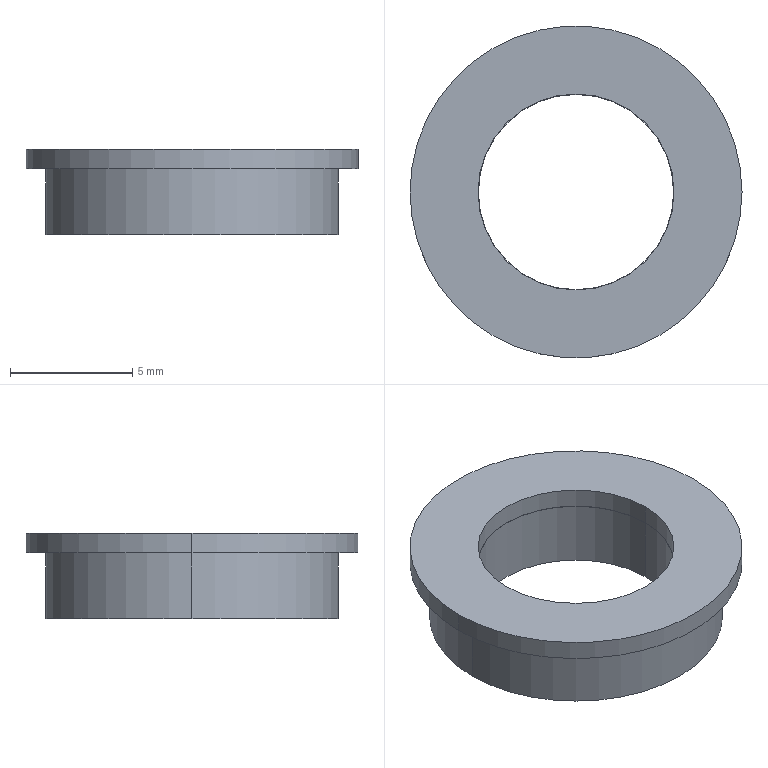Part | SolidWorks | features Extrusion 1, ICE 1 | 1 solid | 12 faces | box 13.6 x 13.6 x 3.5 mm | volume 245.378 mm3 | cylinder 8 | plane 4 | commonest cylinder face diameters 8 x2 8.027 x2 12 x2 13.6 x2
STEP:
#1=CARTESIAN_POINT('',(-4.013,0.,3.5));
#2=VERTEX_POINT('',#1);
#3=CARTESIAN_POINT('',(4.013,0.,3.5));
#4=VERTEX_POINT('',#3);
#5=CARTESIAN_POINT('',(0.,0.,3.5));
#6=DIRECTION('',(0.,0.,1.));
#7=DIRECTION('',(1.,0.,0.));
#8=AXIS2_PLACEMENT_3D('',#5,#6,#7);
#9=CIRCLE('',#8,4.013);
#10=EDGE_CURVE('',#2,#4,#9,.T.);
#11=ORIENTED_EDGE('',*,*,#10,.T.);
#12=CARTESIAN_POINT('',(4.013,0.,2.7));
#13=VERTEX_POINT('',#12);
#14=CARTESIAN_POINT('',(4.013,0.,3.5));
#15=DIRECTION('',(0.,0.,-1.));
#16=VECTOR('',#15,1000.);
#17=LINE('',#14,#16);
#18=EDGE_CURVE('',#4,#13,#17,.T.);
#19=ORIENTED_EDGE('',*,*,#18,.T.);
#20=CARTESIAN_POINT('',(-4.013,0.,2.7));
#21=VERTEX_POINT('',#20);
#22=CARTESIAN_POINT('',(0.,0.,2.7));
#23=DIRECTION('',(0.,0.,-1.));
#24=DIRECTION('',(1.,0.,0.));
#25=AXIS2_PLACEMENT_3D('',#22,#23,#24);
#26=CIRCLE('',#25,4.013);
#27=EDGE_CURVE('',#13,#21,#26,.T.);
#28=ORIENTED_EDGE('',*,*,#27,.T.);
#29=CARTESIAN_POINT('',(-4.013,0.,3.5));
#30=DIRECTION('',(0.,0.,-1.));
#31=VECTOR('',#30,1000.);
#32=LINE('',#29,#31);
#33=EDGE_CURVE('',#2,#21,#32,.T.);
#34=ORIENTED_EDGE('',*,*,#33,.F.);
#35=EDGE_LOOP('',(#11,#19,#28,#34));
#36=FACE_OUTER_BOUND('',#35,.T.);
#37=CARTESIAN_POINT('',(0.,0.,3.5));
#38=DIRECTION('',(0.,0.,-1.));
#39=DIRECTION('',(-1.,0.,0.));
#40=AXIS2_PLACEMENT_3D('',#37,#38,#39);
#41=CYLINDRICAL_SURFACE('',#40,4.013);
#42=ADVANCED_FACE('',(#36),#41,.F.);
#43=CARTESIAN_POINT('',(6.8,0.,3.5));
#44=VERTEX_POINT('',#43);
#45=CARTESIAN_POINT('',(-6.8,0.,3.5));
#46=VERTEX_POINT('',#45);
#47=CARTESIAN_POINT('',(0.,0.,3.5));
#48=DIRECTION('',(0.,0.,1.));
#49=DIRECTION('',(1.,0.,0.));
#50=AXIS2_PLACEMENT_3D('',#47,#48,#49);
#51=CIRCLE('',#50,6.8);
#52=EDGE_CURVE('',#44,#46,#51,.T.);
#53=ORIENTED_EDGE('',*,*,#52,.F.);
#54=CARTESIAN_POINT('',(6.8,0.,2.7));
#55=VERTEX_POINT('',#54);
#56=CARTESIAN_POINT('',(6.8,0.,3.5));
#57=DIRECTION('',(0.,0.,-1.));
#58=VECTOR('',#57,1000.);
#59=LINE('',#56,#58);
#60=EDGE_CURVE('',#44,#55,#59,.T.);
#61=ORIENTED_EDGE('',*,*,#60,.T.);
#62=CARTESIAN_POINT('',(-6.8,0.,2.7));
#63=VERTEX_POINT('',#62);
#64=CARTESIAN_POINT('',(0.,0.,2.7));
#65=DIRECTION('',(0.,0.,1.));
#66=DIRECTION('',(1.,0.,0.));
#67=AXIS2_PLACEMENT_3D('',#64,#65,#66);
#68=CIRCLE('',#67,6.8);
#69=EDGE_CURVE('',#55,#63,#68,.T.);
#70=ORIENTED_EDGE('',*,*,#69,.T.);
#71=CARTESIAN_POINT('',(-6.8,0.,3.5));
#72=DIRECTION('',(0.,0.,-1.));
#73=VECTOR('',#72,1000.);
#74=LINE('',#71,#73);
#75=EDGE_CURVE('',#46,#63,#74,.T.);
#76=ORIENTED_EDGE('',*,*,#75,.F.);
#77=EDGE_LOOP('',(#53,#61,#70,#76));
#78=FACE_OUTER_BOUND('',#77,.T.);
#79=CARTESIAN_POINT('',(0.,0.,3.5));
#80=DIRECTION('',(0.,0.,-1.));
#81=DIRECTION('',(-1.,0.,0.));
#82=AXIS2_PLACEMENT_3D('',#79,#80,#81);
#83=CYLINDRICAL_SURFACE('',#82,6.8);
#84=ADVANCED_FACE('',(#78),#83,.T.);
#85=CARTESIAN_POINT('',(-4.,0.,2.7));
#86=VERTEX_POINT('',#85);
#87=CARTESIAN_POINT('',(4.,0.,2.7));
#88=VERTEX_POINT('',#87);
#89=CARTESIAN_POINT('',(0.,0.,2.7));
#90=DIRECTION('',(0.,0.,1.));
#91=DIRECTION('',(1.,0.,0.));
#92=AXIS2_PLACEMENT_3D('',#89,#90,#91);
#93=CIRCLE('',#92,4.);
#94=EDGE_CURVE('',#86,#88,#93,.T.);
#95=ORIENTED_EDGE('',*,*,#94,.T.);
#96=CARTESIAN_POINT('',(4.,0.,0.));
#97=VERTEX_POINT('',#96);
#98=CARTESIAN_POINT('',(4.,0.,2.7));
#99=DIRECTION('',(0.,0.,-1.));
#100=VECTOR('',#99,1000.);
#101=LINE('',#98,#100);
#102=EDGE_CURVE('',#88,#97,#101,.T.);
#103=ORIENTED_EDGE('',*,*,#102,.T.);
#104=CARTESIAN_POINT('',(-4.,0.,0.));
#105=VERTEX_POINT('',#104);
#106=CARTESIAN_POINT('',(0.,0.,0.));
#107=DIRECTION('',(0.,0.,1.));
#108=DIRECTION('',(1.,0.,0.));
#109=AXIS2_PLACEMENT_3D('',#106,#107,#108);
#110=CIRCLE('',#109,4.);
#111=EDGE_CURVE('',#105,#97,#110,.T.);
#112=ORIENTED_EDGE('',*,*,#111,.F.);
#113=CARTESIAN_POINT('',(-4.,0.,2.7));
#114=DIRECTION('',(0.,0.,-1.));
#115=VECTOR('',#114,1000.);
#116=LINE('',#113,#115);
#117=EDGE_CURVE('',#86,#105,#116,.T.);
#118=ORIENTED_EDGE('',*,*,#117,.F.);
#119=EDGE_LOOP('',(#95,#103,#112,#118));
#120=FACE_OUTER_BOUND('',#119,.T.);
#121=CARTESIAN_POINT('',(0.,0.,2.7));
#122=DIRECTION('',(0.,0.,-1.));
#123=DIRECTION('',(-1.,0.,0.));
#124=AXIS2_PLACEMENT_3D('',#121,#122,#123);
#125=CYLINDRICAL_SURFACE('',#124,4.);
#126=ADVANCED_FACE('',(#120),#125,.F.);
#127=CARTESIAN_POINT('',(6.,0.,2.7));
#128=VERTEX_POINT('',#127);
#129=CARTESIAN_POINT('',(-6.,0.,2.7));
#130=VERTEX_POINT('',#129);
#131=CARTESIAN_POINT('',(0.,0.,2.7));
#132=DIRECTION('',(0.,0.,1.));
#133=DIRECTION('',(1.,0.,0.));
#134=AXIS2_PLACEMENT_3D('',#131,#132,#133);
#135=CIRCLE('',#134,6.);
#136=EDGE_CURVE('',#128,#130,#135,.T.);
#137=ORIENTED_EDGE('',*,*,#136,.F.);
#138=CARTESIAN_POINT('',(6.,0.,0.));
#139=VERTEX_POINT('',#138);
#140=CARTESIAN_POINT('',(6.,0.,2.7));
#141=DIRECTION('',(0.,0.,-1.));
#142=VECTOR('',#141,1000.);
#143=LINE('',#140,#142);
#144=EDGE_CURVE('',#128,#139,#143,.T.);
#145=ORIENTED_EDGE('',*,*,#144,.T.);
#146=CARTESIAN_POINT('',(-6.,0.,0.));
#147=VERTEX_POINT('',#146);
#148=CARTESIAN_POINT('',(0.,0.,0.));
#149=DIRECTION('',(0.,0.,1.));
#150=DIRECTION('',(1.,0.,0.));
#151=AXIS2_PLACEMENT_3D('',#148,#149,#150);
#152=CIRCLE('',#151,6.);
#153=EDGE_CURVE('',#139,#147,#152,.T.);
#154=ORIENTED_EDGE('',*,*,#153,.T.);
#155=CARTESIAN_POINT('',(-6.,0.,2.7));
#156=DIRECTION('',(0.,0.,-1.));
#157=VECTOR('',#156,1000.);
#158=LINE('',#155,#157);
#159=EDGE_CURVE('',#130,#147,#158,.T.);
#160=ORIENTED_EDGE('',*,*,#159,.F.);
#161=EDGE_LOOP('',(#137,#145,#154,#160));
#162=FACE_OUTER_BOUND('',#161,.T.);
#163=CARTESIAN_POINT('',(0.,0.,2.7));
#164=DIRECTION('',(0.,0.,-1.));
#165=DIRECTION('',(-1.,0.,0.));
#166=AXIS2_PLACEMENT_3D('',#163,#164,#165);
#167=CYLINDRICAL_SURFACE('',#166,6.);
#168=ADVANCED_FACE('',(#162),#167,.T.);
#169=CARTESIAN_POINT('',(0.,0.,2.7));
#170=DIRECTION('',(0.,0.,-1.));
#171=DIRECTION('',(1.,0.,0.));
#172=AXIS2_PLACEMENT_3D('',#169,#170,#171);
#173=CIRCLE('',#172,4.013);
#174=EDGE_CURVE('',#21,#13,#173,.T.);
#175=ORIENTED_EDGE('',*,*,#174,.F.);
#176=ORIENTED_EDGE('',*,*,#27,.F.);
#177=EDGE_LOOP('',(#175,#176));
#178=FACE_OUTER_BOUND('',#177,.T.);
#179=ORIENTED_EDGE('',*,*,#94,.F.);
#180=CARTESIAN_POINT('',(0.,0.,2.7));
#181=DIRECTION('',(0.,0.,1.));
#182=DIRECTION('',(1.,0.,0.));
#183=AXIS2_PLACEMENT_3D('',#180,#181,#182);
#184=CIRCLE('',#183,4.);
#185=EDGE_CURVE('',#88,#86,#184,.T.);
#186=ORIENTED_EDGE('',*,*,#185,.F.);
#187=EDGE_LOOP('',(#179,#186));
#188=FACE_BOUND('',#187,.T.);
#189=CARTESIAN_POINT('',(0.,0.,2.7));
#190=DIRECTION('',(0.,0.,1.));
#191=DIRECTION('',(1.,0.,0.));
#192=AXIS2_PLACEMENT_3D('',#189,#190,#191);
#193=PLANE('',#192);
#194=ADVANCED_FACE('',(#178,#188),#193,.T.);
#195=CARTESIAN_POINT('',(0.,0.,0.));
#196=DIRECTION('',(0.,0.,1.));
#197=DIRECTION('',(1.,0.,0.));
#198=AXIS2_PLACEMENT_3D('',#195,#196,#197);
#199=CIRCLE('',#198,6.);
#200=EDGE_CURVE('',#147,#139,#199,.T.);
#201=ORIENTED_EDGE('',*,*,#200,.F.);
#202=ORIENTED_EDGE('',*,*,#153,.F.);
#203=EDGE_LOOP('',(#201,#202));
#204=FACE_OUTER_BOUND('',#203,.T.);
#205=ORIENTED_EDGE('',*,*,#111,.T.);
#206=CARTESIAN_POINT('',(0.,0.,0.));
#207=DIRECTION('',(0.,0.,1.));
#208=DIRECTION('',(1.,0.,0.));
#209=AXIS2_PLACEMENT_3D('',#206,#207,#208);
#210=CIRCLE('',#209,4.);
#211=EDGE_CURVE('',#97,#105,#210,.T.);
#212=ORIENTED_EDGE('',*,*,#211,.T.);
#213=EDGE_LOOP('',(#205,#212));
#214=FACE_BOUND('',#213,.T.);
#215=CARTESIAN_POINT('',(0.,0.,0.));
#216=DIRECTION('',(0.,0.,1.));
#217=DIRECTION('',(1.,0.,0.));
#218=AXIS2_PLACEMENT_3D('',#215,#216,#217);
#219=PLANE('',#218);
#220=ADVANCED_FACE('',(#204,#214),#219,.F.);
#221=ORIENTED_EDGE('',*,*,#144,.F.);
#222=CARTESIAN_POINT('',(0.,0.,2.7));
#223=DIRECTION('',(0.,0.,1.));
#224=DIRECTION('',(1.,0.,0.));
#225=AXIS2_PLACEMENT_3D('',#222,#223,#224);
#226=CIRCLE('',#225,6.);
#227=EDGE_CURVE('',#130,#128,#226,.T.);
#228=ORIENTED_EDGE('',*,*,#227,.F.);
#229=ORIENTED_EDGE('',*,*,#159,.T.);
#230=ORIENTED_EDGE('',*,*,#200,.T.);
#231=EDGE_LOOP('',(#221,#228,#229,#230));
#232=FACE_OUTER_BOUND('',#231,.T.);
#233=CARTESIAN_POINT('',(0.,0.,2.7));
#234=DIRECTION('',(0.,0.,-1.));
#235=DIRECTION('',(-1.,0.,0.));
#236=AXIS2_PLACEMENT_3D('',#233,#234,#235);
#237=CYLINDRICAL_SURFACE('',#236,6.);
#238=ADVANCED_FACE('',(#232),#237,.T.);
#239=ORIENTED_EDGE('',*,*,#102,.F.);
#240=ORIENTED_EDGE('',*,*,#185,.T.);
#241=ORIENTED_EDGE('',*,*,#117,.T.);
#242=ORIENTED_EDGE('',*,*,#211,.F.);
#243=EDGE_LOOP('',(#239,#240,#241,#242));
#244=FACE_OUTER_BOUND('',#243,.T.);
#245=CARTESIAN_POINT('',(0.,0.,2.7));
#246=DIRECTION('',(0.,0.,-1.));
#247=DIRECTION('',(-1.,0.,0.));
#248=AXIS2_PLACEMENT_3D('',#245,#246,#247);
#249=CYLINDRICAL_SURFACE('',#248,4.);
#250=ADVANCED_FACE('',(#244),#249,.F.);
#251=CARTESIAN_POINT('',(0.,0.,2.7));
#252=DIRECTION('',(0.,0.,1.));
#253=DIRECTION('',(1.,0.,0.));
#254=AXIS2_PLACEMENT_3D('',#251,#252,#253);
#255=CIRCLE('',#254,6.8);
#256=EDGE_CURVE('',#63,#55,#255,.T.);
#257=ORIENTED_EDGE('',*,*,#256,.F.);
#258=ORIENTED_EDGE('',*,*,#69,.F.);
#259=EDGE_LOOP('',(#257,#258));
#260=FACE_OUTER_BOUND('',#259,.T.);
#261=ORIENTED_EDGE('',*,*,#227,.T.);
#262=ORIENTED_EDGE('',*,*,#136,.T.);
#263=EDGE_LOOP('',(#261,#262));
#264=FACE_BOUND('',#263,.T.);
#265=CARTESIAN_POINT('',(0.,0.,2.7));
#266=DIRECTION('',(0.,0.,1.));
#267=DIRECTION('',(1.,0.,0.));
#268=AXIS2_PLACEMENT_3D('',#265,#266,#267);
#269=PLANE('',#268);
#270=ADVANCED_FACE('',(#260,#264),#269,.F.);
#271=CARTESIAN_POINT('',(0.,0.,3.5));
#272=DIRECTION('',(0.,0.,1.));
#273=DIRECTION('',(1.,0.,0.));
#274=AXIS2_PLACEMENT_3D('',#271,#272,#273);
#275=CIRCLE('',#274,6.8);
#276=EDGE_CURVE('',#46,#44,#275,.T.);
#277=ORIENTED_EDGE('',*,*,#276,.T.);
#278=ORIENTED_EDGE('',*,*,#52,.T.);
#279=EDGE_LOOP('',(#277,#278));
#280=FACE_OUTER_BOUND('',#279,.T.);
#281=ORIENTED_EDGE('',*,*,#10,.F.);
#282=CARTESIAN_POINT('',(0.,0.,3.5));
#283=DIRECTION('',(0.,0.,1.));
#284=DIRECTION('',(1.,0.,0.));
#285=AXIS2_PLACEMENT_3D('',#282,#283,#284);
#286=CIRCLE('',#285,4.013);
#287=EDGE_CURVE('',#4,#2,#286,.T.);
#288=ORIENTED_EDGE('',*,*,#287,.F.);
#289=EDGE_LOOP('',(#281,#288));
#290=FACE_BOUND('',#289,.T.);
#291=CARTESIAN_POINT('',(0.,0.,3.5));
#292=DIRECTION('',(0.,0.,1.));
#293=DIRECTION('',(1.,0.,0.));
#294=AXIS2_PLACEMENT_3D('',#291,#292,#293);
#295=PLANE('',#294);
#296=ADVANCED_FACE('',(#280,#290),#295,.T.);
#297=ORIENTED_EDGE('',*,*,#60,.F.);
#298=ORIENTED_EDGE('',*,*,#276,.F.);
#299=ORIENTED_EDGE('',*,*,#75,.T.);
#300=ORIENTED_EDGE('',*,*,#256,.T.);
#301=EDGE_LOOP('',(#297,#298,#299,#300));
#302=FACE_OUTER_BOUND('',#301,.T.);
#303=CARTESIAN_POINT('',(0.,0.,3.5));
#304=DIRECTION('',(0.,0.,-1.));
#305=DIRECTION('',(-1.,0.,0.));
#306=AXIS2_PLACEMENT_3D('',#303,#304,#305);
#307=CYLINDRICAL_SURFACE('',#306,6.8);
#308=ADVANCED_FACE('',(#302),#307,.T.);
#309=ORIENTED_EDGE('',*,*,#18,.F.);
#310=ORIENTED_EDGE('',*,*,#287,.T.);
#311=ORIENTED_EDGE('',*,*,#33,.T.);
#312=ORIENTED_EDGE('',*,*,#174,.T.);
#313=EDGE_LOOP('',(#309,#310,#311,#312));
#314=FACE_OUTER_BOUND('',#313,.T.);
#315=CARTESIAN_POINT('',(0.,0.,3.5));
#316=DIRECTION('',(0.,0.,-1.));
#317=DIRECTION('',(-1.,0.,0.));
#318=AXIS2_PLACEMENT_3D('',#315,#316,#317);
#319=CYLINDRICAL_SURFACE('',#318,4.013);
#320=ADVANCED_FACE('',(#314),#319,.F.);
#321=CLOSED_SHELL('',(#42,#84,#126,#168,#194,#220,#238,#250,#270,#296,#308,#320));
#322=MANIFOLD_SOLID_BREP('',#321);
#323=CARTESIAN_POINT('',(0.,0.,0.));
#324=DIRECTION('',(0.,0.,1.));
#325=DIRECTION('',(1.,0.,0.));
#326=AXIS2_PLACEMENT_3D('',#323,#324,#325);
#327=(LENGTH_UNIT()NAMED_UNIT(*)SI_UNIT(.MILLI.,.METRE.));
#328=UNCERTAINTY_MEASURE_WITH_UNIT(LENGTH_MEASURE(0.00001),#327,'','');
#329=(NAMED_UNIT(*)PLANE_ANGLE_UNIT()SI_UNIT($,.RADIAN.));
#330=(NAMED_UNIT(*)SI_UNIT($,.STERADIAN.)SOLID_ANGLE_UNIT());
#331=(GEOMETRIC_REPRESENTATION_CONTEXT(3)GLOBAL_UNCERTAINTY_ASSIGNED_CONTEXT((#328))GLOBAL_UNIT_ASSIGNED_CONTEXT((#327,#329,#330))REPRESENTATION_CONTEXT('',''));
#332=ADVANCED_BREP_SHAPE_REPRESENTATION('',(#322,#326),#331);